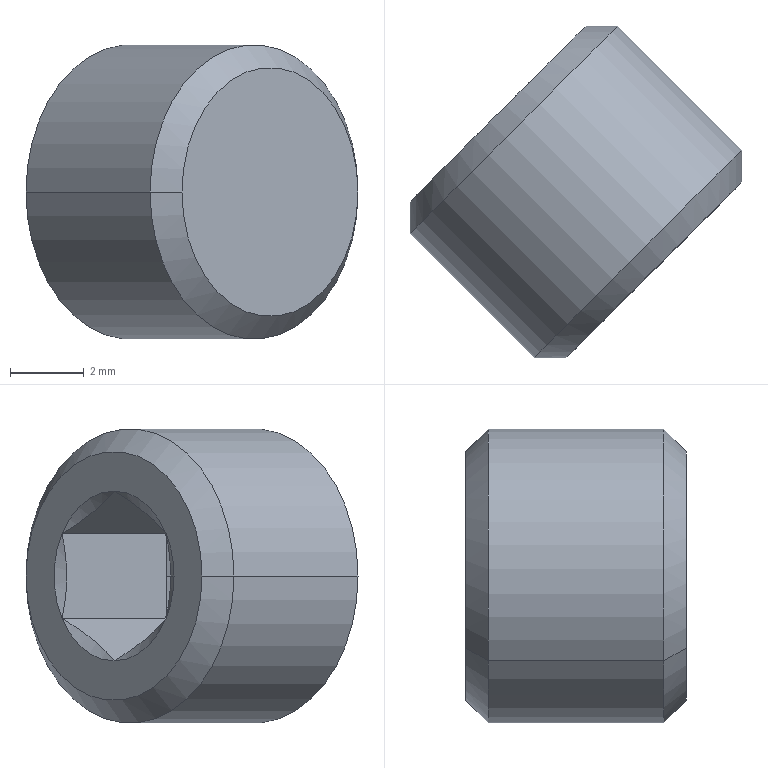Part | SolidWorks | features BaseBody 1 | 1 solid | 29 faces | box 9.032 x 9.032 x 8 mm | volume 229.539 mm3 | plane 14 | cone 13 | cylinder 2 | commonest cylinder face diameters 8 x2
STEP:
#1=CARTESIAN_POINT('',(-17.404,11.748,-237.243));
#2=VERTEX_POINT('',#1);
#3=CARTESIAN_POINT('',(-11.748,17.404,-237.243));
#4=VERTEX_POINT('',#3);
#5=CARTESIAN_POINT('',(-14.576,14.576,-237.243));
#6=DIRECTION('',(-0.7071,0.7071,0.));
#7=DIRECTION('',(-0.7071,-0.7071,0.));
#8=AXIS2_PLACEMENT_3D('',#5,#6,#7);
#9=CIRCLE('',#8,4.);
#10=EDGE_CURVE('',#2,#4,#9,.T.);
#11=ORIENTED_EDGE('',*,*,#10,.T.);
#12=CARTESIAN_POINT('',(-15.123,20.779,-237.243));
#13=VERTEX_POINT('',#12);
#14=CARTESIAN_POINT('',(-11.314,16.971,-237.243));
#15=DIRECTION('',(-0.7071,0.7071,0.));
#16=VECTOR('',#15,1000.);
#17=LINE('',#14,#16);
#18=EDGE_CURVE('',#4,#13,#17,.T.);
#19=ORIENTED_EDGE('',*,*,#18,.T.);
#20=CARTESIAN_POINT('',(-20.779,15.123,-237.243));
#21=VERTEX_POINT('',#20);
#22=CARTESIAN_POINT('',(-17.951,17.951,-237.243));
#23=DIRECTION('',(0.7071,-0.7071,0.));
#24=DIRECTION('',(-0.7071,-0.7071,0.));
#25=AXIS2_PLACEMENT_3D('',#22,#23,#24);
#26=CIRCLE('',#25,4.);
#27=EDGE_CURVE('',#13,#21,#26,.T.);
#28=ORIENTED_EDGE('',*,*,#27,.T.);
#29=CARTESIAN_POINT('',(-16.971,11.314,-237.243));
#30=DIRECTION('',(-0.7071,0.7071,0.));
#31=VECTOR('',#30,1000.);
#32=LINE('',#29,#31);
#33=EDGE_CURVE('',#2,#21,#32,.T.);
#34=ORIENTED_EDGE('',*,*,#33,.F.);
#35=EDGE_LOOP('',(#11,#19,#28,#34));
#36=FACE_OUTER_BOUND('',#35,.T.);
#37=CARTESIAN_POINT('',(-14.142,14.142,-237.243));
#38=DIRECTION('',(-0.7071,0.7071,0.));
#39=DIRECTION('',(-0.7071,-0.7071,0.));
#40=AXIS2_PLACEMENT_3D('',#37,#38,#39);
#41=CYLINDRICAL_SURFACE('',#40,4.);
#42=ADVANCED_FACE('',(#36),#41,.T.);
#43=CARTESIAN_POINT('',(-15.99,20.779,-237.243));
#44=VERTEX_POINT('',#43);
#45=CARTESIAN_POINT('',(-20.779,15.99,-237.243));
#46=VERTEX_POINT('',#45);
#47=CARTESIAN_POINT('',(-18.385,18.385,-237.243));
#48=DIRECTION('',(0.7071,-0.7071,0.));
#49=DIRECTION('',(0.7071,0.7071,0.));
#50=AXIS2_PLACEMENT_3D('',#47,#48,#49);
#51=CIRCLE('',#50,3.387);
#52=EDGE_CURVE('',#44,#46,#51,.T.);
#53=ORIENTED_EDGE('',*,*,#52,.T.);
#54=CARTESIAN_POINT('',(-20.779,15.123,-237.243));
#55=DIRECTION('',(0.,-1.,0.));
#56=VECTOR('',#55,1000.);
#57=LINE('',#54,#56);
#58=EDGE_CURVE('',#46,#21,#57,.T.);
#59=ORIENTED_EDGE('',*,*,#58,.T.);
#60=ORIENTED_EDGE('',*,*,#27,.F.);
#61=CARTESIAN_POINT('',(-15.123,20.779,-237.243));
#62=DIRECTION('',(1.,0.,0.));
#63=VECTOR('',#62,1000.);
#64=LINE('',#61,#63);
#65=EDGE_CURVE('',#44,#13,#64,.T.);
#66=ORIENTED_EDGE('',*,*,#65,.F.);
#67=EDGE_LOOP('',(#53,#59,#60,#66));
#68=FACE_OUTER_BOUND('',#67,.T.);
#69=CARTESIAN_POINT('',(-17.951,17.951,-237.243));
#70=DIRECTION('',(0.7071,-0.7071,0.));
#71=DIRECTION('',(0.7071,0.7071,0.));
#72=AXIS2_PLACEMENT_3D('',#69,#70,#71);
#73=CONICAL_SURFACE('',#72,4.,0.7854);
#74=ADVANCED_FACE('',(#68),#73,.T.);
#75=CARTESIAN_POINT('',(-16.537,11.748,-237.243));
#76=VERTEX_POINT('',#75);
#77=CARTESIAN_POINT('',(-11.748,16.537,-237.243));
#78=VERTEX_POINT('',#77);
#79=CARTESIAN_POINT('',(-14.142,14.142,-237.243));
#80=DIRECTION('',(-0.7071,0.7071,0.));
#81=DIRECTION('',(-0.7071,-0.7071,0.));
#82=AXIS2_PLACEMENT_3D('',#79,#80,#81);
#83=CIRCLE('',#82,3.386);
#84=EDGE_CURVE('',#76,#78,#83,.T.);
#85=ORIENTED_EDGE('',*,*,#84,.T.);
#86=CARTESIAN_POINT('',(-11.748,17.404,-237.243));
#87=DIRECTION('',(0.,1.,0.));
#88=VECTOR('',#87,1000.);
#89=LINE('',#86,#88);
#90=EDGE_CURVE('',#78,#4,#89,.T.);
#91=ORIENTED_EDGE('',*,*,#90,.T.);
#92=ORIENTED_EDGE('',*,*,#10,.F.);
#93=CARTESIAN_POINT('',(-17.404,11.748,-237.243));
#94=DIRECTION('',(-1.,0.,0.));
#95=VECTOR('',#94,1000.);
#96=LINE('',#93,#95);
#97=EDGE_CURVE('',#76,#2,#96,.T.);
#98=ORIENTED_EDGE('',*,*,#97,.F.);
#99=EDGE_LOOP('',(#85,#91,#92,#98));
#100=FACE_OUTER_BOUND('',#99,.T.);
#101=CARTESIAN_POINT('',(-14.576,14.576,-237.243));
#102=DIRECTION('',(-0.7071,0.7071,0.));
#103=DIRECTION('',(-0.7071,-0.7071,0.));
#104=AXIS2_PLACEMENT_3D('',#101,#102,#103);
#105=CONICAL_SURFACE('',#104,4.,0.7854);
#106=ADVANCED_FACE('',(#100),#105,.T.);
#107=CARTESIAN_POINT('',(-19.673,16.844,-237.243));
#108=VERTEX_POINT('',#107);
#109=CARTESIAN_POINT('',(-19.799,16.971,-236.088));
#110=VERTEX_POINT('',#109);
#111=CARTESIAN_POINT('',(-19.673,16.844,-237.243));
#112=CARTESIAN_POINT('',(-19.673,16.844,-237.047));
#113=CARTESIAN_POINT('',(-19.685,16.856,-236.851));
#114=CARTESIAN_POINT('',(-19.729,16.9,-236.466));
#115=CARTESIAN_POINT('',(-19.761,16.932,-236.276));
#116=CARTESIAN_POINT('',(-19.799,16.971,-236.088));
#117=B_SPLINE_CURVE_WITH_KNOTS('',3,(#111,#112,#113,#114,#115,#116),.UNSPECIFIED.,.F.,.F.,(4,2,4),(0.001168,0.00175,0.002332),.UNSPECIFIED.);
#118=EDGE_CURVE('',#108,#110,#117,.T.);
#119=ORIENTED_EDGE('',*,*,#118,.F.);
#120=CARTESIAN_POINT('',(-20.018,16.752,-237.243));
#121=VERTEX_POINT('',#120);
#122=CARTESIAN_POINT('',(-20.018,16.752,-237.243));
#123=DIRECTION('',(-0.9659,-0.2588,0.));
#124=VECTOR('',#123,1000.);
#125=LINE('',#122,#124);
#126=EDGE_CURVE('',#108,#121,#125,.T.);
#127=ORIENTED_EDGE('',*,*,#126,.T.);
#128=CARTESIAN_POINT('',(-18.385,18.385,-237.243));
#129=DIRECTION('',(-0.7071,0.7071,0.));
#130=DIRECTION('',(-0.7071,-0.7071,0.));
#131=AXIS2_PLACEMENT_3D('',#128,#129,#130);
#132=CIRCLE('',#131,2.309);
#133=EDGE_CURVE('',#121,#110,#132,.T.);
#134=ORIENTED_EDGE('',*,*,#133,.T.);
#135=EDGE_LOOP('',(#119,#127,#134));
#136=FACE_OUTER_BOUND('',#135,.T.);
#137=CARTESIAN_POINT('',(-18.385,18.385,-237.243));
#138=DIRECTION('',(-0.7071,0.7071,0.));
#139=DIRECTION('',(-0.7071,-0.7071,0.));
#140=AXIS2_PLACEMENT_3D('',#137,#138,#139);
#141=CONICAL_SURFACE('',#140,2.309,1.047);
#142=ADVANCED_FACE('',(#136),#141,.F.);
#143=CARTESIAN_POINT('',(-14.614,14.614,-237.243));
#144=VERTEX_POINT('',#143);
#145=CARTESIAN_POINT('',(-17.189,13.923,-237.243));
#146=VERTEX_POINT('',#145);
#147=CARTESIAN_POINT('',(-17.189,13.923,-237.243));
#148=DIRECTION('',(-0.9659,-0.2588,0.));
#149=VECTOR('',#148,1000.);
#150=LINE('',#147,#149);
#151=EDGE_CURVE('',#144,#146,#150,.T.);
#152=ORIENTED_EDGE('',*,*,#151,.F.);
#153=CARTESIAN_POINT('',(-13.923,17.189,-237.243));
#154=VERTEX_POINT('',#153);
#155=CARTESIAN_POINT('',(-13.923,17.189,-237.243));
#156=DIRECTION('',(0.2588,0.9659,0.));
#157=VECTOR('',#156,1000.);
#158=LINE('',#155,#157);
#159=EDGE_CURVE('',#144,#154,#158,.T.);
#160=ORIENTED_EDGE('',*,*,#159,.T.);
#161=CARTESIAN_POINT('',(-14.142,16.971,-238.397));
#162=VERTEX_POINT('',#161);
#163=CARTESIAN_POINT('',(-15.556,15.556,-237.243));
#164=DIRECTION('',(0.7071,-0.7071,0.));
#165=DIRECTION('',(-0.7071,-0.7071,0.));
#166=AXIS2_PLACEMENT_3D('',#163,#164,#165);
#167=CIRCLE('',#166,2.309);
#168=EDGE_CURVE('',#162,#154,#167,.T.);
#169=ORIENTED_EDGE('',*,*,#168,.F.);
#170=CARTESIAN_POINT('',(-15.556,15.556,-239.552));
#171=VERTEX_POINT('',#170);
#172=CARTESIAN_POINT('',(-15.556,15.556,-237.243));
#173=DIRECTION('',(0.7071,-0.7071,0.));
#174=DIRECTION('',(-0.7071,-0.7071,0.));
#175=AXIS2_PLACEMENT_3D('',#172,#173,#174);
#176=CIRCLE('',#175,2.309);
#177=EDGE_CURVE('',#171,#162,#176,.T.);
#178=ORIENTED_EDGE('',*,*,#177,.F.);
#179=CARTESIAN_POINT('',(-16.971,14.142,-238.397));
#180=VERTEX_POINT('',#179);
#181=CARTESIAN_POINT('',(-15.556,15.556,-237.243));
#182=DIRECTION('',(0.7071,-0.7071,0.));
#183=DIRECTION('',(-0.7071,-0.7071,0.));
#184=AXIS2_PLACEMENT_3D('',#181,#182,#183);
#185=CIRCLE('',#184,2.309);
#186=EDGE_CURVE('',#180,#171,#185,.T.);
#187=ORIENTED_EDGE('',*,*,#186,.F.);
#188=CARTESIAN_POINT('',(-15.556,15.556,-237.243));
#189=DIRECTION('',(0.7071,-0.7071,0.));
#190=DIRECTION('',(-0.7071,-0.7071,0.));
#191=AXIS2_PLACEMENT_3D('',#188,#189,#190);
#192=CIRCLE('',#191,2.309);
#193=EDGE_CURVE('',#146,#180,#192,.T.);
#194=ORIENTED_EDGE('',*,*,#193,.F.);
#195=EDGE_LOOP('',(#152,#160,#169,#178,#187,#194));
#196=FACE_OUTER_BOUND('',#195,.T.);
#197=CARTESIAN_POINT('',(-15.556,15.556,-237.243));
#198=DIRECTION('',(-0.7071,0.7071,0.));
#199=DIRECTION('',(-0.7071,-0.7071,0.));
#200=AXIS2_PLACEMENT_3D('',#197,#198,#199);
#201=CONICAL_SURFACE('',#200,2.309,1.047);
#202=ADVANCED_FACE('',(#196),#201,.F.);
#203=ORIENTED_EDGE('',*,*,#18,.F.);
#204=CARTESIAN_POINT('',(-14.576,14.576,-237.243));
#205=DIRECTION('',(-0.7071,0.7071,0.));
#206=DIRECTION('',(-0.7071,-0.7071,0.));
#207=AXIS2_PLACEMENT_3D('',#204,#205,#206);
#208=CIRCLE('',#207,4.);
#209=EDGE_CURVE('',#4,#2,#208,.T.);
#210=ORIENTED_EDGE('',*,*,#209,.T.);
#211=ORIENTED_EDGE('',*,*,#33,.T.);
#212=CARTESIAN_POINT('',(-17.951,17.951,-237.243));
#213=DIRECTION('',(0.7071,-0.7071,0.));
#214=DIRECTION('',(-0.7071,-0.7071,0.));
#215=AXIS2_PLACEMENT_3D('',#212,#213,#214);
#216=CIRCLE('',#215,4.);
#217=EDGE_CURVE('',#21,#13,#216,.T.);
#218=ORIENTED_EDGE('',*,*,#217,.T.);
#219=EDGE_LOOP('',(#203,#210,#211,#218));
#220=FACE_OUTER_BOUND('',#219,.T.);
#221=CARTESIAN_POINT('',(-14.142,14.142,-237.243));
#222=DIRECTION('',(-0.7071,0.7071,0.));
#223=DIRECTION('',(-0.7071,-0.7071,0.));
#224=AXIS2_PLACEMENT_3D('',#221,#222,#223);
#225=CYLINDRICAL_SURFACE('',#224,4.);
#226=ADVANCED_FACE('',(#220),#225,.T.);
#227=ORIENTED_EDGE('',*,*,#58,.F.);
#228=CARTESIAN_POINT('',(-18.385,18.385,-237.243));
#229=DIRECTION('',(0.7071,-0.7071,0.));
#230=DIRECTION('',(0.7071,0.7071,0.));
#231=AXIS2_PLACEMENT_3D('',#228,#229,#230);
#232=CIRCLE('',#231,3.387);
#233=EDGE_CURVE('',#46,#44,#232,.T.);
#234=ORIENTED_EDGE('',*,*,#233,.T.);
#235=ORIENTED_EDGE('',*,*,#65,.T.);
#236=ORIENTED_EDGE('',*,*,#217,.F.);
#237=EDGE_LOOP('',(#227,#234,#235,#236));
#238=FACE_OUTER_BOUND('',#237,.T.);
#239=CARTESIAN_POINT('',(-17.951,17.951,-237.243));
#240=DIRECTION('',(0.7071,-0.7071,0.));
#241=DIRECTION('',(0.7071,0.7071,0.));
#242=AXIS2_PLACEMENT_3D('',#239,#240,#241);
#243=CONICAL_SURFACE('',#242,4.,0.7854);
#244=ADVANCED_FACE('',(#238),#243,.T.);
#245=ORIENTED_EDGE('',*,*,#90,.F.);
#246=CARTESIAN_POINT('',(-14.142,14.142,-237.243));
#247=DIRECTION('',(-0.7071,0.7071,0.));
#248=DIRECTION('',(-0.7071,-0.7071,0.));
#249=AXIS2_PLACEMENT_3D('',#246,#247,#248);
#250=CIRCLE('',#249,3.386);
#251=EDGE_CURVE('',#78,#76,#250,.T.);
#252=ORIENTED_EDGE('',*,*,#251,.T.);
#253=ORIENTED_EDGE('',*,*,#97,.T.);
#254=ORIENTED_EDGE('',*,*,#209,.F.);
#255=EDGE_LOOP('',(#245,#252,#253,#254));
#256=FACE_OUTER_BOUND('',#255,.T.);
#257=CARTESIAN_POINT('',(-14.576,14.576,-237.243));
#258=DIRECTION('',(-0.7071,0.7071,0.));
#259=DIRECTION('',(-0.7071,-0.7071,0.));
#260=AXIS2_PLACEMENT_3D('',#257,#258,#259);
#261=CONICAL_SURFACE('',#260,4.,0.7854);
#262=ADVANCED_FACE('',(#256),#261,.T.);
#263=ORIENTED_EDGE('',*,*,#52,.F.);
#264=ORIENTED_EDGE('',*,*,#233,.F.);
#265=EDGE_LOOP('',(#263,#264));
#266=FACE_OUTER_BOUND('',#265,.T.);
#267=CARTESIAN_POINT('',(-18.385,18.385,-234.933));
#268=VERTEX_POINT('',#267);
#269=CARTESIAN_POINT('',(-16.971,19.799,-236.088));
#270=VERTEX_POINT('',#269);
#271=CARTESIAN_POINT('',(-18.385,18.385,-237.243));
#272=DIRECTION('',(-0.7071,0.7071,0.));
#273=DIRECTION('',(-0.7071,-0.7071,0.));
#274=AXIS2_PLACEMENT_3D('',#271,#272,#273);
#275=CIRCLE('',#274,2.309);
#276=EDGE_CURVE('',#268,#270,#275,.T.);
#277=ORIENTED_EDGE('',*,*,#276,.F.);
#278=CARTESIAN_POINT('',(-18.385,18.385,-237.243));
#279=DIRECTION('',(-0.7071,0.7071,0.));
#280=DIRECTION('',(-0.7071,-0.7071,0.));
#281=AXIS2_PLACEMENT_3D('',#278,#279,#280);
#282=CIRCLE('',#281,2.309);
#283=EDGE_CURVE('',#110,#268,#282,.T.);
#284=ORIENTED_EDGE('',*,*,#283,.F.);
#285=ORIENTED_EDGE('',*,*,#133,.F.);
#286=CARTESIAN_POINT('',(-19.799,16.971,-238.397));
#287=VERTEX_POINT('',#286);
#288=CARTESIAN_POINT('',(-18.385,18.385,-237.243));
#289=DIRECTION('',(-0.7071,0.7071,0.));
#290=DIRECTION('',(-0.7071,-0.7071,0.));
#291=AXIS2_PLACEMENT_3D('',#288,#289,#290);
#292=CIRCLE('',#291,2.309);
#293=EDGE_CURVE('',#287,#121,#292,.T.);
#294=ORIENTED_EDGE('',*,*,#293,.F.);
#295=CARTESIAN_POINT('',(-18.385,18.385,-239.552));
#296=VERTEX_POINT('',#295);
#297=CARTESIAN_POINT('',(-18.385,18.385,-237.243));
#298=DIRECTION('',(-0.7071,0.7071,0.));
#299=DIRECTION('',(-0.7071,-0.7071,0.));
#300=AXIS2_PLACEMENT_3D('',#297,#298,#299);
#301=CIRCLE('',#300,2.309);
#302=EDGE_CURVE('',#296,#287,#301,.T.);
#303=ORIENTED_EDGE('',*,*,#302,.F.);
#304=CARTESIAN_POINT('',(-16.971,19.799,-238.397));
#305=VERTEX_POINT('',#304);
#306=CARTESIAN_POINT('',(-18.385,18.385,-237.243));
#307=DIRECTION('',(-0.7071,0.7071,0.));
#308=DIRECTION('',(-0.7071,-0.7071,0.));
#309=AXIS2_PLACEMENT_3D('',#306,#307,#308);
#310=CIRCLE('',#309,2.309);
#311=EDGE_CURVE('',#305,#296,#310,.T.);
#312=ORIENTED_EDGE('',*,*,#311,.F.);
#313=CARTESIAN_POINT('',(-18.385,18.385,-237.243));
#314=DIRECTION('',(-0.7071,0.7071,0.));
#315=DIRECTION('',(-0.7071,-0.7071,0.));
#316=AXIS2_PLACEMENT_3D('',#313,#314,#315);
#317=CIRCLE('',#316,2.309);
#318=EDGE_CURVE('',#270,#305,#317,.T.);
#319=ORIENTED_EDGE('',*,*,#318,.F.);
#320=EDGE_LOOP('',(#277,#284,#285,#294,#303,#312,#319));
#321=FACE_BOUND('',#320,.T.);
#322=CARTESIAN_POINT('',(-18.385,18.385,-237.243));
#323=DIRECTION('',(0.7071,-0.7071,0.));
#324=DIRECTION('',(0.7071,0.7071,0.));
#325=AXIS2_PLACEMENT_3D('',#322,#323,#324);
#326=PLANE('',#325);
#327=ADVANCED_FACE('',(#266,#321),#326,.F.);
#328=ORIENTED_EDGE('',*,*,#84,.F.);
#329=ORIENTED_EDGE('',*,*,#251,.F.);
#330=EDGE_LOOP('',(#328,#329));
#331=FACE_OUTER_BOUND('',#330,.T.);
#332=CARTESIAN_POINT('',(-14.142,14.142,-240.629));
#333=DIRECTION('',(-0.7071,0.7071,0.));
#334=DIRECTION('',(-0.7071,-0.7071,0.));
#335=AXIS2_PLACEMENT_3D('',#332,#333,#334);
#336=PLANE('',#335);
#337=ADVANCED_FACE('',(#331),#336,.F.);
#338=CARTESIAN_POINT('',(-16.971,19.799,-236.088));
#339=CARTESIAN_POINT('',(-16.894,19.722,-236.465));
#340=CARTESIAN_POINT('',(-16.844,19.673,-236.848));
#341=CARTESIAN_POINT('',(-16.844,19.673,-237.637));
#342=CARTESIAN_POINT('',(-16.894,19.722,-238.02));
#343=CARTESIAN_POINT('',(-16.971,19.799,-238.397));
#344=B_SPLINE_CURVE_WITH_KNOTS('',3,(#338,#339,#340,#341,#342,#343),.UNSPECIFIED.,.F.,.F.,(4,2,4),(-0.001168,0.,0.001168),.UNSPECIFIED.);
#345=EDGE_CURVE('',#270,#305,#344,.T.);
#346=ORIENTED_EDGE('',*,*,#345,.F.);
#347=ORIENTED_EDGE('',*,*,#318,.T.);
#348=EDGE_LOOP('',(#346,#347));
#349=FACE_OUTER_BOUND('',#348,.T.);
#350=CARTESIAN_POINT('',(-18.385,18.385,-237.243));
#351=DIRECTION('',(-0.7071,0.7071,0.));
#352=DIRECTION('',(-0.7071,-0.7071,0.));
#353=AXIS2_PLACEMENT_3D('',#350,#351,#352);
#354=CONICAL_SURFACE('',#353,2.309,1.047);
#355=ADVANCED_FACE('',(#349),#354,.F.);
#356=ORIENTED_EDGE('',*,*,#276,.T.);
#357=CARTESIAN_POINT('',(-18.385,18.385,-234.933));
#358=CARTESIAN_POINT('',(-18.077,18.539,-235.122));
#359=CARTESIAN_POINT('',(-17.793,18.724,-235.313));
#360=CARTESIAN_POINT('',(-17.432,19.084,-235.608));
#361=CARTESIAN_POINT('',(-17.324,19.217,-235.706));
#362=CARTESIAN_POINT('',(-17.132,19.496,-235.898));
#363=CARTESIAN_POINT('',(-17.048,19.645,-235.993));
#364=CARTESIAN_POINT('',(-16.971,19.799,-236.088));
#365=B_SPLINE_CURVE_WITH_KNOTS('',3,(#357,#358,#359,#360,#361,#362,#363,#364),.UNSPECIFIED.,.F.,.F.,(4,2,2,4),(0.,0.001166,0.001749,0.002332),.UNSPECIFIED.);
#366=EDGE_CURVE('',#268,#270,#365,.T.);
#367=ORIENTED_EDGE('',*,*,#366,.F.);
#368=EDGE_LOOP('',(#356,#367));
#369=FACE_OUTER_BOUND('',#368,.T.);
#370=CARTESIAN_POINT('',(-18.385,18.385,-237.243));
#371=DIRECTION('',(-0.7071,0.7071,0.));
#372=DIRECTION('',(-0.7071,-0.7071,0.));
#373=AXIS2_PLACEMENT_3D('',#370,#371,#372);
#374=CONICAL_SURFACE('',#373,2.309,1.047);
#375=ADVANCED_FACE('',(#369),#374,.F.);
#376=ORIENTED_EDGE('',*,*,#283,.T.);
#377=CARTESIAN_POINT('',(-19.799,16.971,-236.088));
#378=CARTESIAN_POINT('',(-19.491,17.125,-235.899));
#379=CARTESIAN_POINT('',(-19.208,17.31,-235.708));
#380=CARTESIAN_POINT('',(-18.847,17.67,-235.413));
#381=CARTESIAN_POINT('',(-18.739,17.802,-235.315));
#382=CARTESIAN_POINT('',(-18.547,18.082,-235.123));
#383=CARTESIAN_POINT('',(-18.462,18.231,-235.028));
#384=CARTESIAN_POINT('',(-18.385,18.385,-234.933));
#385=B_SPLINE_CURVE_WITH_KNOTS('',3,(#377,#378,#379,#380,#381,#382,#383,#384),.UNSPECIFIED.,.F.,.F.,(4,2,2,4),(0.,0.001166,0.001749,0.002332),.UNSPECIFIED.);
#386=EDGE_CURVE('',#110,#268,#385,.T.);
#387=ORIENTED_EDGE('',*,*,#386,.F.);
#388=EDGE_LOOP('',(#376,#387));
#389=FACE_OUTER_BOUND('',#388,.T.);
#390=CARTESIAN_POINT('',(-18.385,18.385,-237.243));
#391=DIRECTION('',(-0.7071,0.7071,0.));
#392=DIRECTION('',(-0.7071,-0.7071,0.));
#393=AXIS2_PLACEMENT_3D('',#390,#391,#392);
#394=CONICAL_SURFACE('',#393,2.309,1.047);
#395=ADVANCED_FACE('',(#389),#394,.F.);
#396=ORIENTED_EDGE('',*,*,#126,.F.);
#397=CARTESIAN_POINT('',(-19.799,16.971,-238.397));
#398=CARTESIAN_POINT('',(-19.722,16.893,-238.019));
#399=CARTESIAN_POINT('',(-19.673,16.844,-237.636));
#400=CARTESIAN_POINT('',(-19.673,16.844,-237.243));
#401=B_SPLINE_CURVE_WITH_KNOTS('',3,(#397,#398,#399,#400),.UNSPECIFIED.,.F.,.F.,(4,4),(0.,0.001168),.UNSPECIFIED.);
#402=EDGE_CURVE('',#287,#108,#401,.T.);
#403=ORIENTED_EDGE('',*,*,#402,.F.);
#404=ORIENTED_EDGE('',*,*,#293,.T.);
#405=EDGE_LOOP('',(#396,#403,#404));
#406=FACE_OUTER_BOUND('',#405,.T.);
#407=CARTESIAN_POINT('',(-18.385,18.385,-237.243));
#408=DIRECTION('',(-0.7071,0.7071,0.));
#409=DIRECTION('',(-0.7071,-0.7071,0.));
#410=AXIS2_PLACEMENT_3D('',#407,#408,#409);
#411=CONICAL_SURFACE('',#410,2.309,1.047);
#412=ADVANCED_FACE('',(#406),#411,.F.);
#413=ORIENTED_EDGE('',*,*,#302,.T.);
#414=CARTESIAN_POINT('',(-18.385,18.385,-239.552));
#415=CARTESIAN_POINT('',(-18.539,18.077,-239.363));
#416=CARTESIAN_POINT('',(-18.724,17.793,-239.172));
#417=CARTESIAN_POINT('',(-19.084,17.432,-238.878));
#418=CARTESIAN_POINT('',(-19.217,17.324,-238.779));
#419=CARTESIAN_POINT('',(-19.496,17.132,-238.587));
#420=CARTESIAN_POINT('',(-19.645,17.048,-238.492));
#421=CARTESIAN_POINT('',(-19.799,16.971,-238.397));
#422=B_SPLINE_CURVE_WITH_KNOTS('',3,(#414,#415,#416,#417,#418,#419,#420,#421),.UNSPECIFIED.,.F.,.F.,(4,2,2,4),(0.,0.001166,0.001749,0.002332),.UNSPECIFIED.);
#423=EDGE_CURVE('',#296,#287,#422,.T.);
#424=ORIENTED_EDGE('',*,*,#423,.F.);
#425=EDGE_LOOP('',(#413,#424));
#426=FACE_OUTER_BOUND('',#425,.T.);
#427=CARTESIAN_POINT('',(-18.385,18.385,-237.243));
#428=DIRECTION('',(-0.7071,0.7071,0.));
#429=DIRECTION('',(-0.7071,-0.7071,0.));
#430=AXIS2_PLACEMENT_3D('',#427,#428,#429);
#431=CONICAL_SURFACE('',#430,2.309,1.047);
#432=ADVANCED_FACE('',(#426),#431,.F.);
#433=ORIENTED_EDGE('',*,*,#311,.T.);
#434=CARTESIAN_POINT('',(-16.971,19.799,-238.397));
#435=CARTESIAN_POINT('',(-17.125,19.491,-238.586));
#436=CARTESIAN_POINT('',(-17.31,19.208,-238.777));
#437=CARTESIAN_POINT('',(-17.67,18.847,-239.072));
#438=CARTESIAN_POINT('',(-17.802,18.739,-239.17));
#439=CARTESIAN_POINT('',(-18.082,18.547,-239.362));
#440=CARTESIAN_POINT('',(-18.231,18.462,-239.458));
#441=CARTESIAN_POINT('',(-18.385,18.385,-239.552));
#442=B_SPLINE_CURVE_WITH_KNOTS('',3,(#434,#435,#436,#437,#438,#439,#440,#441),.UNSPECIFIED.,.F.,.F.,(4,2,2,4),(0.,0.001166,0.001749,0.002332),.UNSPECIFIED.);
#443=EDGE_CURVE('',#305,#296,#442,.T.);
#444=ORIENTED_EDGE('',*,*,#443,.F.);
#445=EDGE_LOOP('',(#433,#444));
#446=FACE_OUTER_BOUND('',#445,.T.);
#447=CARTESIAN_POINT('',(-18.385,18.385,-237.243));
#448=DIRECTION('',(-0.7071,0.7071,0.));
#449=DIRECTION('',(-0.7071,-0.7071,0.));
#450=AXIS2_PLACEMENT_3D('',#447,#448,#449);
#451=CONICAL_SURFACE('',#450,2.309,1.047);
#452=ADVANCED_FACE('',(#446),#451,.F.);
#453=CARTESIAN_POINT('',(-14.142,16.971,-236.088));
#454=VERTEX_POINT('',#453);
#455=CARTESIAN_POINT('',(-16.971,19.799,-236.088));
#456=DIRECTION('',(0.7071,-0.7071,0.));
#457=VECTOR('',#456,1000.);
#458=LINE('',#455,#457);
#459=EDGE_CURVE('',#270,#454,#458,.T.);
#460=ORIENTED_EDGE('',*,*,#459,.T.);
#461=CARTESIAN_POINT('',(-15.556,15.556,-234.933));
#462=VERTEX_POINT('',#461);
#463=CARTESIAN_POINT('',(-14.142,16.971,-236.088));
#464=DIRECTION('',(-0.6124,-0.6124,0.5));
#465=VECTOR('',#464,1000.);
#466=LINE('',#463,#465);
#467=EDGE_CURVE('',#454,#462,#466,.T.);
#468=ORIENTED_EDGE('',*,*,#467,.T.);
#469=CARTESIAN_POINT('',(-15.556,15.556,-234.933));
#470=DIRECTION('',(-0.7071,0.7071,0.));
#471=VECTOR('',#470,1000.);
#472=LINE('',#469,#471);
#473=EDGE_CURVE('',#462,#268,#472,.T.);
#474=ORIENTED_EDGE('',*,*,#473,.T.);
#475=ORIENTED_EDGE('',*,*,#366,.T.);
#476=EDGE_LOOP('',(#460,#468,#474,#475));
#477=FACE_OUTER_BOUND('',#476,.T.);
#478=CARTESIAN_POINT('',(-14.142,16.971,-236.088));
#479=DIRECTION('',(-0.3536,-0.3536,-0.866));
#480=DIRECTION('',(-0.9258,0.,0.378));
#481=AXIS2_PLACEMENT_3D('',#478,#479,#480);
#482=PLANE('',#481);
#483=ADVANCED_FACE('',(#477),#482,.T.);
#484=ORIENTED_EDGE('',*,*,#473,.F.);
#485=CARTESIAN_POINT('',(-16.971,14.142,-236.088));
#486=VERTEX_POINT('',#485);
#487=CARTESIAN_POINT('',(-15.556,15.556,-234.933));
#488=DIRECTION('',(-0.6124,-0.6124,-0.5));
#489=VECTOR('',#488,1000.);
#490=LINE('',#487,#489);
#491=EDGE_CURVE('',#462,#486,#490,.T.);
#492=ORIENTED_EDGE('',*,*,#491,.T.);
#493=CARTESIAN_POINT('',(-16.971,14.142,-236.088));
#494=DIRECTION('',(-0.7071,0.7071,0.));
#495=VECTOR('',#494,1000.);
#496=LINE('',#493,#495);
#497=EDGE_CURVE('',#486,#110,#496,.T.);
#498=ORIENTED_EDGE('',*,*,#497,.T.);
#499=ORIENTED_EDGE('',*,*,#386,.T.);
#500=EDGE_LOOP('',(#484,#492,#498,#499));
#501=FACE_OUTER_BOUND('',#500,.T.);
#502=CARTESIAN_POINT('',(-15.556,15.556,-234.933));
#503=DIRECTION('',(0.3536,0.3536,-0.866));
#504=DIRECTION('',(-0.9258,0.,-0.378));
#505=AXIS2_PLACEMENT_3D('',#502,#503,#504);
#506=PLANE('',#505);
#507=ADVANCED_FACE('',(#501),#506,.T.);
#508=ORIENTED_EDGE('',*,*,#497,.F.);
#509=CARTESIAN_POINT('',(-16.971,14.142,-236.088));
#510=DIRECTION('',(0.,0.,-1.));
#511=VECTOR('',#510,1000.);
#512=LINE('',#509,#511);
#513=EDGE_CURVE('',#486,#180,#512,.T.);
#514=ORIENTED_EDGE('',*,*,#513,.T.);
#515=CARTESIAN_POINT('',(-16.971,14.142,-238.397));
#516=DIRECTION('',(-0.7071,0.7071,0.));
#517=VECTOR('',#516,1000.);
#518=LINE('',#515,#517);
#519=EDGE_CURVE('',#180,#287,#518,.T.);
#520=ORIENTED_EDGE('',*,*,#519,.T.);
#521=ORIENTED_EDGE('',*,*,#402,.T.);
#522=ORIENTED_EDGE('',*,*,#118,.T.);
#523=EDGE_LOOP('',(#508,#514,#520,#521,#522));
#524=FACE_OUTER_BOUND('',#523,.T.);
#525=CARTESIAN_POINT('',(-16.971,14.142,-236.088));
#526=DIRECTION('',(0.7071,0.7071,0.));
#527=DIRECTION('',(-0.7071,0.7071,0.));
#528=AXIS2_PLACEMENT_3D('',#525,#526,#527);
#529=PLANE('',#528);
#530=ADVANCED_FACE('',(#524),#529,.T.);
#531=ORIENTED_EDGE('',*,*,#519,.F.);
#532=CARTESIAN_POINT('',(-16.971,14.142,-238.397));
#533=DIRECTION('',(0.6124,0.6124,-0.5));
#534=VECTOR('',#533,1000.);
#535=LINE('',#532,#534);
#536=EDGE_CURVE('',#180,#171,#535,.T.);
#537=ORIENTED_EDGE('',*,*,#536,.T.);
#538=CARTESIAN_POINT('',(-15.556,15.556,-239.552));
#539=DIRECTION('',(-0.7071,0.7071,0.));
#540=VECTOR('',#539,1000.);
#541=LINE('',#538,#540);
#542=EDGE_CURVE('',#171,#296,#541,.T.);
#543=ORIENTED_EDGE('',*,*,#542,.T.);
#544=ORIENTED_EDGE('',*,*,#423,.T.);
#545=EDGE_LOOP('',(#531,#537,#543,#544));
#546=FACE_OUTER_BOUND('',#545,.T.);
#547=CARTESIAN_POINT('',(-16.971,14.142,-238.397));
#548=DIRECTION('',(0.3536,0.3536,0.866));
#549=DIRECTION('',(0.9258,0.,-0.378));
#550=AXIS2_PLACEMENT_3D('',#547,#548,#549);
#551=PLANE('',#550);
#552=ADVANCED_FACE('',(#546),#551,.T.);
#553=ORIENTED_EDGE('',*,*,#542,.F.);
#554=CARTESIAN_POINT('',(-15.556,15.556,-239.552));
#555=DIRECTION('',(0.6124,0.6124,0.5));
#556=VECTOR('',#555,1000.);
#557=LINE('',#554,#556);
#558=EDGE_CURVE('',#171,#162,#557,.T.);
#559=ORIENTED_EDGE('',*,*,#558,.T.);
#560=CARTESIAN_POINT('',(-14.142,16.971,-238.397));
#561=DIRECTION('',(-0.7071,0.7071,0.));
#562=VECTOR('',#561,1000.);
#563=LINE('',#560,#562);
#564=EDGE_CURVE('',#162,#305,#563,.T.);
#565=ORIENTED_EDGE('',*,*,#564,.T.);
#566=ORIENTED_EDGE('',*,*,#443,.T.);
#567=EDGE_LOOP('',(#553,#559,#565,#566));
#568=FACE_OUTER_BOUND('',#567,.T.);
#569=CARTESIAN_POINT('',(-15.556,15.556,-239.552));
#570=DIRECTION('',(-0.3536,-0.3536,0.866));
#571=DIRECTION('',(0.9258,0.,0.378));
#572=AXIS2_PLACEMENT_3D('',#569,#570,#571);
#573=PLANE('',#572);
#574=ADVANCED_FACE('',(#568),#573,.T.);
#575=CARTESIAN_POINT('',(-15.556,15.556,-237.243));
#576=DIRECTION('',(0.7071,-0.7071,0.));
#577=DIRECTION('',(-0.7071,-0.7071,0.));
#578=AXIS2_PLACEMENT_3D('',#575,#576,#577);
#579=CIRCLE('',#578,2.309);
#580=EDGE_CURVE('',#454,#462,#579,.T.);
#581=ORIENTED_EDGE('',*,*,#580,.T.);
#582=ORIENTED_EDGE('',*,*,#467,.F.);
#583=EDGE_LOOP('',(#581,#582));
#584=FACE_OUTER_BOUND('',#583,.T.);
#585=CARTESIAN_POINT('',(-15.556,15.556,-237.243));
#586=DIRECTION('',(0.7071,-0.7071,0.));
#587=DIRECTION('',(0.7071,0.7071,0.));
#588=AXIS2_PLACEMENT_3D('',#585,#586,#587);
#589=PLANE('',#588);
#590=ADVANCED_FACE('',(#584),#589,.T.);
#591=ORIENTED_EDGE('',*,*,#564,.F.);
#592=CARTESIAN_POINT('',(-14.142,16.971,-238.397));
#593=DIRECTION('',(0.,0.,1.));
#594=VECTOR('',#593,1000.);
#595=LINE('',#592,#594);
#596=EDGE_CURVE('',#162,#454,#595,.T.);
#597=ORIENTED_EDGE('',*,*,#596,.T.);
#598=ORIENTED_EDGE('',*,*,#459,.F.);
#599=ORIENTED_EDGE('',*,*,#345,.T.);
#600=EDGE_LOOP('',(#591,#597,#598,#599));
#601=FACE_OUTER_BOUND('',#600,.T.);
#602=CARTESIAN_POINT('',(-14.142,16.971,-238.397));
#603=DIRECTION('',(-0.7071,-0.7071,0.));
#604=DIRECTION('',(0.7071,-0.7071,0.));
#605=AXIS2_PLACEMENT_3D('',#602,#603,#604);
#606=PLANE('',#605);
#607=ADVANCED_FACE('',(#601),#606,.T.);
#608=CARTESIAN_POINT('',(-15.556,15.556,-237.243));
#609=DIRECTION('',(0.7071,-0.7071,0.));
#610=DIRECTION('',(-0.7071,-0.7071,0.));
#611=AXIS2_PLACEMENT_3D('',#608,#609,#610);
#612=CIRCLE('',#611,2.309);
#613=EDGE_CURVE('',#462,#486,#612,.T.);
#614=ORIENTED_EDGE('',*,*,#613,.T.);
#615=ORIENTED_EDGE('',*,*,#491,.F.);
#616=EDGE_LOOP('',(#614,#615));
#617=FACE_OUTER_BOUND('',#616,.T.);
#618=CARTESIAN_POINT('',(-15.556,15.556,-237.243));
#619=DIRECTION('',(0.7071,-0.7071,0.));
#620=DIRECTION('',(0.7071,0.7071,0.));
#621=AXIS2_PLACEMENT_3D('',#618,#619,#620);
#622=PLANE('',#621);
#623=ADVANCED_FACE('',(#617),#622,.T.);
#624=ORIENTED_EDGE('',*,*,#513,.F.);
#625=CARTESIAN_POINT('',(-15.556,15.556,-237.243));
#626=DIRECTION('',(0.7071,-0.7071,0.));
#627=DIRECTION('',(-0.7071,-0.7071,0.));
#628=AXIS2_PLACEMENT_3D('',#625,#626,#627);
#629=CIRCLE('',#628,2.309);
#630=EDGE_CURVE('',#486,#146,#629,.T.);
#631=ORIENTED_EDGE('',*,*,#630,.T.);
#632=ORIENTED_EDGE('',*,*,#193,.T.);
#633=EDGE_LOOP('',(#624,#631,#632));
#634=FACE_OUTER_BOUND('',#633,.T.);
#635=CARTESIAN_POINT('',(-15.556,15.556,-237.243));
#636=DIRECTION('',(0.7071,-0.7071,0.));
#637=DIRECTION('',(0.7071,0.7071,0.));
#638=AXIS2_PLACEMENT_3D('',#635,#636,#637);
#639=PLANE('',#638);
#640=ADVANCED_FACE('',(#634),#639,.T.);
#641=ORIENTED_EDGE('',*,*,#186,.T.);
#642=ORIENTED_EDGE('',*,*,#536,.F.);
#643=EDGE_LOOP('',(#641,#642));
#644=FACE_OUTER_BOUND('',#643,.T.);
#645=CARTESIAN_POINT('',(-15.556,15.556,-237.243));
#646=DIRECTION('',(0.7071,-0.7071,0.));
#647=DIRECTION('',(0.7071,0.7071,0.));
#648=AXIS2_PLACEMENT_3D('',#645,#646,#647);
#649=PLANE('',#648);
#650=ADVANCED_FACE('',(#644),#649,.T.);
#651=ORIENTED_EDGE('',*,*,#177,.T.);
#652=ORIENTED_EDGE('',*,*,#558,.F.);
#653=EDGE_LOOP('',(#651,#652));
#654=FACE_OUTER_BOUND('',#653,.T.);
#655=CARTESIAN_POINT('',(-15.556,15.556,-237.243));
#656=DIRECTION('',(0.7071,-0.7071,0.));
#657=DIRECTION('',(0.7071,0.7071,0.));
#658=AXIS2_PLACEMENT_3D('',#655,#656,#657);
#659=PLANE('',#658);
#660=ADVANCED_FACE('',(#654),#659,.T.);
#661=ORIENTED_EDGE('',*,*,#159,.F.);
#662=ORIENTED_EDGE('',*,*,#151,.T.);
#663=ORIENTED_EDGE('',*,*,#630,.F.);
#664=ORIENTED_EDGE('',*,*,#613,.F.);
#665=ORIENTED_EDGE('',*,*,#580,.F.);
#666=CARTESIAN_POINT('',(-15.556,15.556,-237.243));
#667=DIRECTION('',(0.7071,-0.7071,0.));
#668=DIRECTION('',(-0.7071,-0.7071,0.));
#669=AXIS2_PLACEMENT_3D('',#666,#667,#668);
#670=CIRCLE('',#669,2.309);
#671=EDGE_CURVE('',#154,#454,#670,.T.);
#672=ORIENTED_EDGE('',*,*,#671,.F.);
#673=EDGE_LOOP('',(#661,#662,#663,#664,#665,#672));
#674=FACE_OUTER_BOUND('',#673,.T.);
#675=CARTESIAN_POINT('',(-15.556,15.556,-237.243));
#676=DIRECTION('',(-0.7071,0.7071,0.));
#677=DIRECTION('',(-0.7071,-0.7071,0.));
#678=AXIS2_PLACEMENT_3D('',#675,#676,#677);
#679=CONICAL_SURFACE('',#678,2.309,1.047);
#680=ADVANCED_FACE('',(#674),#679,.F.);
#681=ORIENTED_EDGE('',*,*,#596,.F.);
#682=ORIENTED_EDGE('',*,*,#168,.T.);
#683=ORIENTED_EDGE('',*,*,#671,.T.);
#684=EDGE_LOOP('',(#681,#682,#683));
#685=FACE_OUTER_BOUND('',#684,.T.);
#686=CARTESIAN_POINT('',(-15.556,15.556,-237.243));
#687=DIRECTION('',(0.7071,-0.7071,0.));
#688=DIRECTION('',(0.7071,0.7071,0.));
#689=AXIS2_PLACEMENT_3D('',#686,#687,#688);
#690=PLANE('',#689);
#691=ADVANCED_FACE('',(#685),#690,.T.);
#692=CLOSED_SHELL('',(#42,#74,#106,#142,#202,#226,#244,#262,#327,#337,#355,#375,#395,#412,#432,#452,#483,#507,#530,#552,#574,#590,#607,#623,#640,#650,#660,#680,#691));
#693=MANIFOLD_SOLID_BREP('',#692);
#694=CARTESIAN_POINT('',(0.,0.,0.));
#695=DIRECTION('',(0.,0.,1.));
#696=DIRECTION('',(1.,0.,0.));
#697=AXIS2_PLACEMENT_3D('',#694,#695,#696);
#698=(LENGTH_UNIT()NAMED_UNIT(*)SI_UNIT(.MILLI.,.METRE.));
#699=UNCERTAINTY_MEASURE_WITH_UNIT(LENGTH_MEASURE(0.00001),#698,'','');
#700=(NAMED_UNIT(*)PLANE_ANGLE_UNIT()SI_UNIT($,.RADIAN.));
#701=(NAMED_UNIT(*)SI_UNIT($,.STERADIAN.)SOLID_ANGLE_UNIT());
#702=(GEOMETRIC_REPRESENTATION_CONTEXT(3)GLOBAL_UNCERTAINTY_ASSIGNED_CONTEXT((#699))GLOBAL_UNIT_ASSIGNED_CONTEXT((#698,#700,#701))REPRESENTATION_CONTEXT('',''));
#703=ADVANCED_BREP_SHAPE_REPRESENTATION('',(#693,#697),#702);